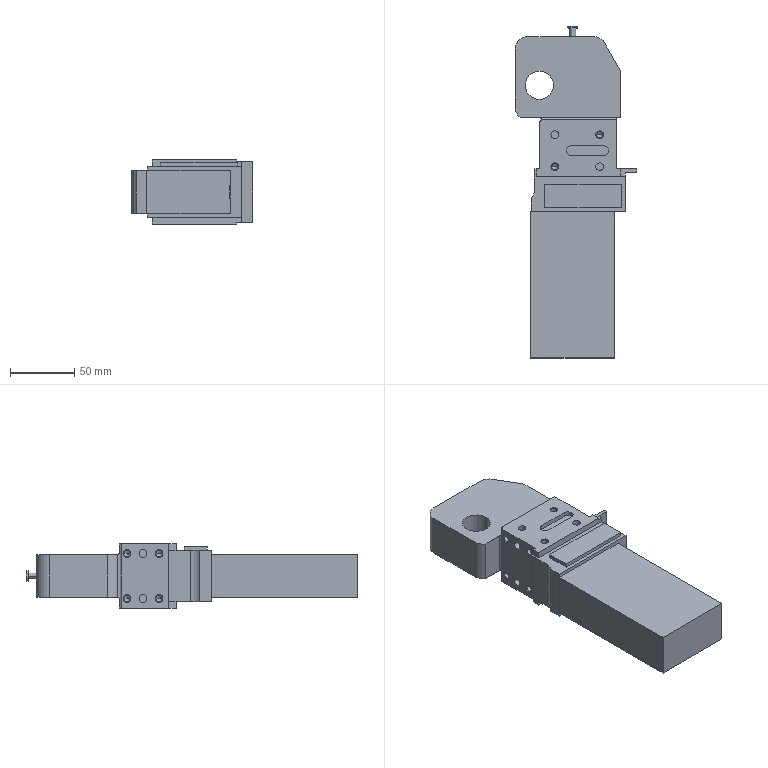Part | NX | features BREP 1 | 1 solid | 200 faces | box 95 x 258.75 x 50 mm | volume 616254 mm3 | cylinder 69 | cone 68 | plane 63 | commonest cylinder face diameters 4.917 x26 6 x16 4.134 x4 8 x4 8.566 x4 20 x4